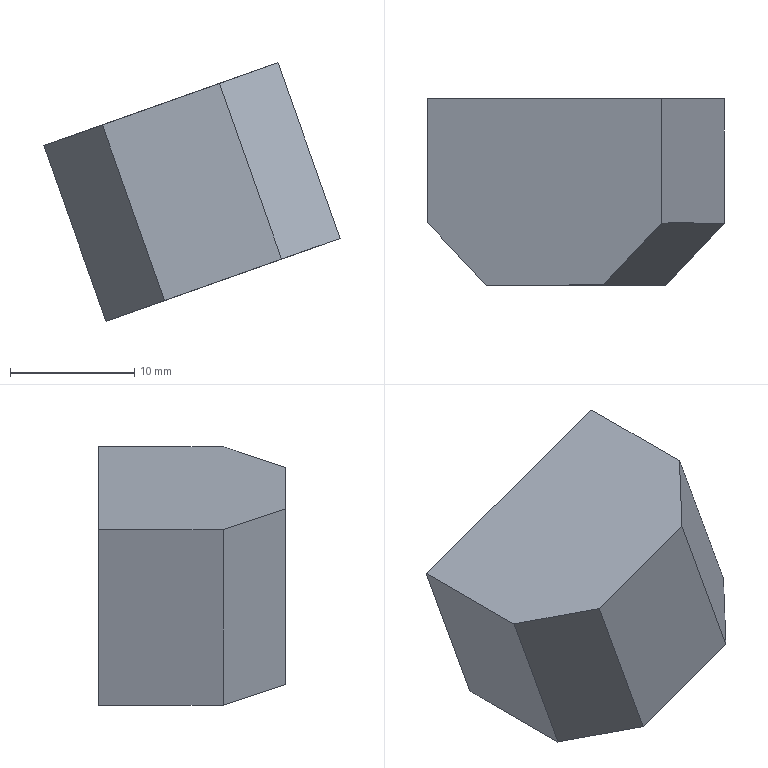Part | STEP file | RACK1-INSERT_id678_x_t | 1 solid | 8 faces | box 23.86 x 15 x 20.816 mm | volume 4125 mm3 | plane 8
STEP:
#1=CARTESIAN_POINT('',(-91.684,-174.472,-96.948));
#2=VERTEX_POINT('',#1);
#3=CARTESIAN_POINT('',(-96.691,-174.472,-82.808));
#4=VERTEX_POINT('',#3);
#5=CARTESIAN_POINT('',(-91.684,-174.472,-96.948));
#6=DIRECTION('',(-0.3338,0.,0.9426));
#7=VECTOR('',#6,1.);
#8=LINE('',#5,#7);
#9=EDGE_CURVE('',#2,#4,#8,.T.);
#10=ORIENTED_EDGE('',*,*,#9,.F.);
#11=CARTESIAN_POINT('',(-82.257,-174.472,-93.61));
#12=VERTEX_POINT('',#11);
#13=CARTESIAN_POINT('',(59.139,-174.472,-43.539));
#14=DIRECTION('',(0.9426,0.,0.3338));
#15=VECTOR('',#14,1.);
#16=LINE('',#13,#15);
#17=EDGE_CURVE('',#2,#12,#16,.T.);
#18=ORIENTED_EDGE('',*,*,#17,.T.);
#19=CARTESIAN_POINT('',(-87.264,-174.472,-79.47));
#20=VERTEX_POINT('',#19);
#21=CARTESIAN_POINT('',(-87.264,-174.472,-79.47));
#22=DIRECTION('',(0.3338,0.,-0.9426));
#23=VECTOR('',#22,1.);
#24=LINE('',#21,#23);
#25=EDGE_CURVE('',#20,#12,#24,.T.);
#26=ORIENTED_EDGE('',*,*,#25,.F.);
#27=CARTESIAN_POINT('',(54.132,-174.472,-29.399));
#28=DIRECTION('',(0.9426,0.,0.3338));
#29=VECTOR('',#28,1.);
#30=LINE('',#27,#29);
#31=EDGE_CURVE('',#4,#20,#30,.T.);
#32=ORIENTED_EDGE('',*,*,#31,.F.);
#33=EDGE_LOOP('',(#10,#18,#26,#32));
#34=FACE_OUTER_BOUND('',#33,.T.);
#35=CARTESIAN_POINT('',(-96.397,-174.472,-98.617));
#36=DIRECTION('',(0.,-1.,0.));
#37=DIRECTION('',(0.,0.,-1.));
#38=AXIS2_PLACEMENT_3D('',#35,#36,#37);
#39=PLANE('',#38);
#40=ADVANCED_FACE('',(#34),#39,.T.);
#41=CARTESIAN_POINT('',(-77.544,-169.472,-91.941));
#42=VERTEX_POINT('',#41);
#43=CARTESIAN_POINT('',(-82.257,-174.472,-93.61));
#44=DIRECTION('',(0.6665,0.7071,0.236));
#45=VECTOR('',#44,1.);
#46=LINE('',#43,#45);
#47=EDGE_CURVE('',#12,#42,#46,.T.);
#48=ORIENTED_EDGE('',*,*,#47,.T.);
#49=CARTESIAN_POINT('',(-82.551,-169.472,-77.801));
#50=VERTEX_POINT('',#49);
#51=CARTESIAN_POINT('',(-77.544,-169.472,-91.941));
#52=DIRECTION('',(0.3338,0.,-0.9426));
#53=VECTOR('',#52,1.);
#54=LINE('',#51,#53);
#55=EDGE_CURVE('',#50,#42,#54,.T.);
#56=ORIENTED_EDGE('',*,*,#55,.F.);
#57=CARTESIAN_POINT('',(-87.264,-174.472,-79.47));
#58=DIRECTION('',(0.6665,0.7071,0.236));
#59=VECTOR('',#58,1.);
#60=LINE('',#57,#59);
#61=EDGE_CURVE('',#20,#50,#60,.T.);
#62=ORIENTED_EDGE('',*,*,#61,.F.);
#63=ORIENTED_EDGE('',*,*,#25,.T.);
#64=EDGE_LOOP('',(#48,#56,#62,#63));
#65=FACE_OUTER_BOUND('',#64,.T.);
#66=CARTESIAN_POINT('',(-77.544,-169.472,-91.941));
#67=DIRECTION('',(0.6665,-0.7071,0.236));
#68=DIRECTION('',(0.7277,0.6859,0.));
#69=AXIS2_PLACEMENT_3D('',#66,#67,#68);
#70=PLANE('',#69);
#71=ADVANCED_FACE('',(#65),#70,.T.);
#72=CARTESIAN_POINT('',(-96.397,-169.472,-98.617));
#73=VERTEX_POINT('',#72);
#74=CARTESIAN_POINT('',(-96.397,-169.472,-98.617));
#75=DIRECTION('',(0.6665,-0.7071,0.236));
#76=VECTOR('',#75,1.);
#77=LINE('',#74,#76);
#78=EDGE_CURVE('',#73,#2,#77,.T.);
#79=ORIENTED_EDGE('',*,*,#78,.T.);
#80=ORIENTED_EDGE('',*,*,#9,.T.);
#81=CARTESIAN_POINT('',(-101.404,-169.472,-84.477));
#82=VERTEX_POINT('',#81);
#83=CARTESIAN_POINT('',(-101.404,-169.472,-84.477));
#84=DIRECTION('',(0.6665,-0.7071,0.236));
#85=VECTOR('',#84,1.);
#86=LINE('',#83,#85);
#87=EDGE_CURVE('',#82,#4,#86,.T.);
#88=ORIENTED_EDGE('',*,*,#87,.F.);
#89=CARTESIAN_POINT('',(-96.397,-169.472,-98.617));
#90=DIRECTION('',(-0.3338,0.,0.9426));
#91=VECTOR('',#90,1.);
#92=LINE('',#89,#91);
#93=EDGE_CURVE('',#73,#82,#92,.T.);
#94=ORIENTED_EDGE('',*,*,#93,.F.);
#95=EDGE_LOOP('',(#79,#80,#88,#94));
#96=FACE_OUTER_BOUND('',#95,.T.);
#97=CARTESIAN_POINT('',(-91.684,-174.472,-96.948));
#98=DIRECTION('',(-0.6665,-0.7071,-0.236));
#99=DIRECTION('',(0.7277,-0.6859,0.));
#100=AXIS2_PLACEMENT_3D('',#97,#98,#99);
#101=PLANE('',#100);
#102=ADVANCED_FACE('',(#96),#101,.T.);
#103=CARTESIAN_POINT('',(-96.397,-159.472,-98.617));
#104=VERTEX_POINT('',#103);
#105=CARTESIAN_POINT('',(-101.404,-159.472,-84.477));
#106=VERTEX_POINT('',#105);
#107=CARTESIAN_POINT('',(-96.397,-159.472,-98.617));
#108=DIRECTION('',(-0.3338,0.,0.9426));
#109=VECTOR('',#108,1.);
#110=LINE('',#107,#109);
#111=EDGE_CURVE('',#104,#106,#110,.T.);
#112=ORIENTED_EDGE('',*,*,#111,.F.);
#113=CARTESIAN_POINT('',(-96.397,-166.472,-98.617));
#114=DIRECTION('',(0.,-1.,0.));
#115=VECTOR('',#114,1.);
#116=LINE('',#113,#115);
#117=EDGE_CURVE('',#104,#73,#116,.T.);
#118=ORIENTED_EDGE('',*,*,#117,.T.);
#119=ORIENTED_EDGE('',*,*,#93,.T.);
#120=CARTESIAN_POINT('',(-101.404,-166.472,-84.477));
#121=DIRECTION('',(0.,-1.,0.));
#122=VECTOR('',#121,1.);
#123=LINE('',#120,#122);
#124=EDGE_CURVE('',#106,#82,#123,.T.);
#125=ORIENTED_EDGE('',*,*,#124,.F.);
#126=EDGE_LOOP('',(#112,#118,#119,#125));
#127=FACE_OUTER_BOUND('',#126,.T.);
#128=CARTESIAN_POINT('',(-96.397,-159.472,-98.617));
#129=DIRECTION('',(-0.9426,0.,-0.3338));
#130=DIRECTION('',(-0.3338,0.,0.9426));
#131=AXIS2_PLACEMENT_3D('',#128,#129,#130);
#132=PLANE('',#131);
#133=ADVANCED_FACE('',(#127),#132,.T.);
#134=ORIENTED_EDGE('',*,*,#87,.T.);
#135=ORIENTED_EDGE('',*,*,#31,.T.);
#136=ORIENTED_EDGE('',*,*,#61,.T.);
#137=CARTESIAN_POINT('',(-82.551,-159.472,-77.801));
#138=VERTEX_POINT('',#137);
#139=CARTESIAN_POINT('',(-82.551,-174.472,-77.801));
#140=DIRECTION('',(0.,-1.,0.));
#141=VECTOR('',#140,1.);
#142=LINE('',#139,#141);
#143=EDGE_CURVE('',#138,#50,#142,.T.);
#144=ORIENTED_EDGE('',*,*,#143,.F.);
#145=CARTESIAN_POINT('',(-101.404,-159.472,-84.477));
#146=DIRECTION('',(0.9426,0.,0.3338));
#147=VECTOR('',#146,1.);
#148=LINE('',#145,#147);
#149=EDGE_CURVE('',#106,#138,#148,.T.);
#150=ORIENTED_EDGE('',*,*,#149,.F.);
#151=ORIENTED_EDGE('',*,*,#124,.T.);
#152=EDGE_LOOP('',(#134,#135,#136,#144,#150,#151));
#153=FACE_OUTER_BOUND('',#152,.T.);
#154=CARTESIAN_POINT('',(54.132,-166.472,-29.399));
#155=DIRECTION('',(-0.3338,0.,0.9426));
#156=DIRECTION('',(0.9426,0.,0.3338));
#157=AXIS2_PLACEMENT_3D('',#154,#155,#156);
#158=PLANE('',#157);
#159=ADVANCED_FACE('',(#153),#158,.T.);
#160=ORIENTED_EDGE('',*,*,#55,.T.);
#161=CARTESIAN_POINT('',(-77.544,-159.472,-91.941));
#162=VERTEX_POINT('',#161);
#163=CARTESIAN_POINT('',(-77.544,-166.472,-91.941));
#164=DIRECTION('',(0.,1.,0.));
#165=VECTOR('',#164,1.);
#166=LINE('',#163,#165);
#167=EDGE_CURVE('',#42,#162,#166,.T.);
#168=ORIENTED_EDGE('',*,*,#167,.T.);
#169=CARTESIAN_POINT('',(-82.551,-159.472,-77.801));
#170=DIRECTION('',(0.3338,0.,-0.9426));
#171=VECTOR('',#170,1.);
#172=LINE('',#169,#171);
#173=EDGE_CURVE('',#138,#162,#172,.T.);
#174=ORIENTED_EDGE('',*,*,#173,.F.);
#175=ORIENTED_EDGE('',*,*,#143,.T.);
#176=EDGE_LOOP('',(#160,#168,#174,#175));
#177=FACE_OUTER_BOUND('',#176,.T.);
#178=CARTESIAN_POINT('',(-77.544,-174.472,-91.941));
#179=DIRECTION('',(0.9426,0.,0.3338));
#180=DIRECTION('',(0.3338,0.,-0.9426));
#181=AXIS2_PLACEMENT_3D('',#178,#179,#180);
#182=PLANE('',#181);
#183=ADVANCED_FACE('',(#177),#182,.T.);
#184=ORIENTED_EDGE('',*,*,#117,.F.);
#185=CARTESIAN_POINT('',(-77.544,-159.472,-91.941));
#186=DIRECTION('',(-0.9426,0.,-0.3338));
#187=VECTOR('',#186,1.);
#188=LINE('',#185,#187);
#189=EDGE_CURVE('',#162,#104,#188,.T.);
#190=ORIENTED_EDGE('',*,*,#189,.F.);
#191=ORIENTED_EDGE('',*,*,#167,.F.);
#192=ORIENTED_EDGE('',*,*,#47,.F.);
#193=ORIENTED_EDGE('',*,*,#17,.F.);
#194=ORIENTED_EDGE('',*,*,#78,.F.);
#195=EDGE_LOOP('',(#184,#190,#191,#192,#193,#194));
#196=FACE_OUTER_BOUND('',#195,.T.);
#197=CARTESIAN_POINT('',(59.139,-166.472,-43.539));
#198=DIRECTION('',(-0.3338,0.,0.9426));
#199=DIRECTION('',(0.9426,0.,0.3338));
#200=AXIS2_PLACEMENT_3D('',#197,#198,#199);
#201=PLANE('',#200);
#202=ADVANCED_FACE('',(#196),#201,.F.);
#203=ORIENTED_EDGE('',*,*,#173,.T.);
#204=ORIENTED_EDGE('',*,*,#189,.T.);
#205=ORIENTED_EDGE('',*,*,#111,.T.);
#206=ORIENTED_EDGE('',*,*,#149,.T.);
#207=EDGE_LOOP('',(#203,#204,#205,#206));
#208=FACE_OUTER_BOUND('',#207,.T.);
#209=CARTESIAN_POINT('',(-77.544,-159.472,-91.941));
#210=DIRECTION('',(0.,1.,0.));
#211=DIRECTION('',(0.,0.,1.));
#212=AXIS2_PLACEMENT_3D('',#209,#210,#211);
#213=PLANE('',#212);
#214=ADVANCED_FACE('',(#208),#213,.T.);
#215=CLOSED_SHELL('',(#40,#71,#102,#133,#159,#183,#202,#214));
#216=MANIFOLD_SOLID_BREP('',#215);
#217=(LENGTH_UNIT()NAMED_UNIT(*)SI_UNIT(.MILLI.,.METRE.));
#218=UNCERTAINTY_MEASURE_WITH_UNIT(LENGTH_MEASURE(0.00002),#217,'','');
#219=(NAMED_UNIT(*)PLANE_ANGLE_UNIT()SI_UNIT($,.RADIAN.));
#220=PLANE_ANGLE_MEASURE_WITH_UNIT(PLANE_ANGLE_MEASURE(0.01745),#219);
#221=DIMENSIONAL_EXPONENTS(0.,0.,0.,0.,0.,0.,0.);
#222=(CONVERSION_BASED_UNIT('DEGREE',#220)NAMED_UNIT(#221)PLANE_ANGLE_UNIT());
#223=(NAMED_UNIT(*)SI_UNIT($,.STERADIAN.)SOLID_ANGLE_UNIT());
#224=(GEOMETRIC_REPRESENTATION_CONTEXT(3)GLOBAL_UNCERTAINTY_ASSIGNED_CONTEXT((#218))GLOBAL_UNIT_ASSIGNED_CONTEXT((#217,#222,#223))REPRESENTATION_CONTEXT('',''));
#225=ADVANCED_BREP_SHAPE_REPRESENTATION('',(#216),#224);